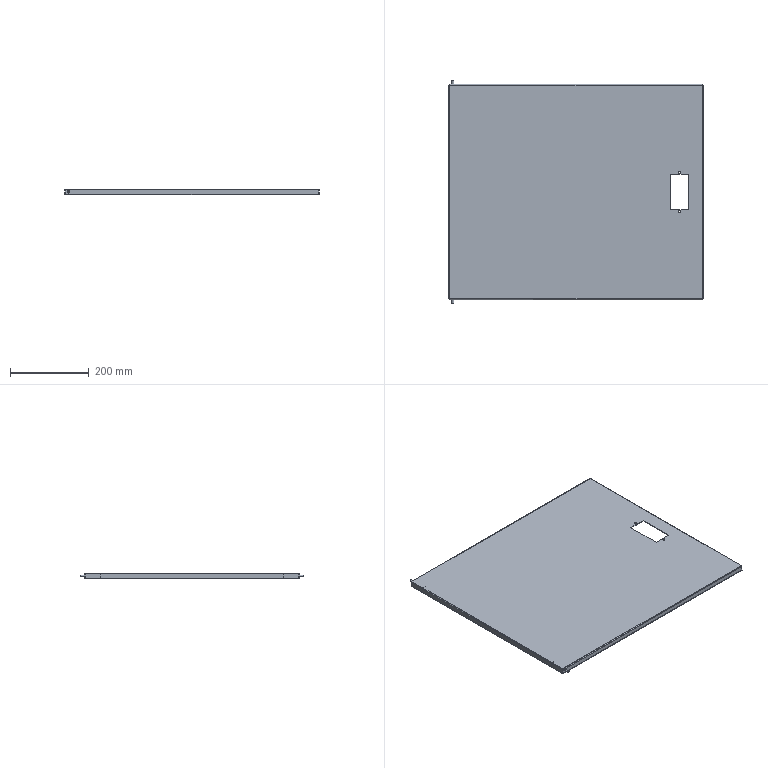Part | SolidWorks | features ICE 5, FlatPattern 1, Helix 1, MirrorPattern 1, SMBaseFlange 1, SMMiteredFlange 1, SheetMetal 1, Sweep 1 | 1 solid | 112 faces | box 647 x 568 x 15 mm | volume 618702 mm3 | plane 61 | cylinder 29 | spline 22 | commonest cylinder face diameters 1.473 x9 4.473 x8 4.8 x4 5 x4 6 x4